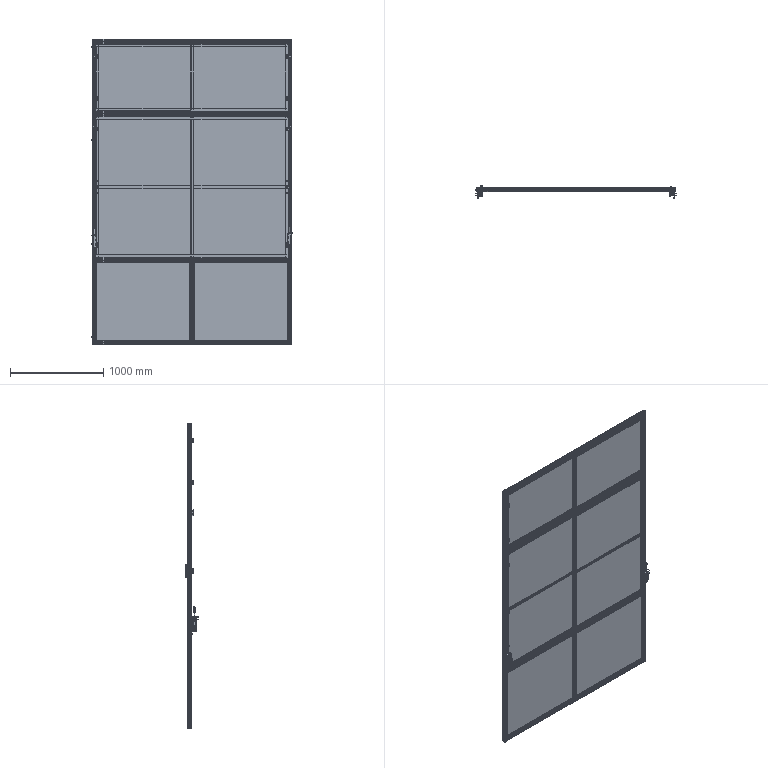Part | SolidWorks | 391 solids | 20690 faces | volume 46606535 mm3 | plane 11291 | cylinder 5390 | cone 2651 | spline 820 | torus 446 | sphere 92 | commonest cylinder face diameters 1 x492 5 x452 2 x370 2.5 x356 11 x268 8 x230